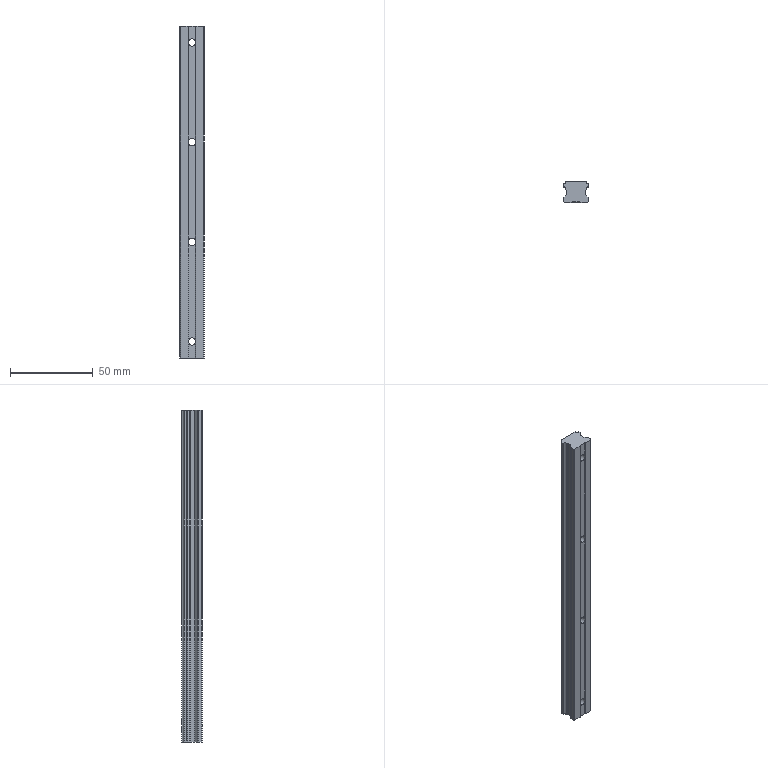Part | STEP file | 11-EG15_RAIL_170CW11 | 1 solid | 70 faces | box 15 x 12.5 x 200 mm | volume 31138 mm3 | cylinder 34 | plane 28 | cone 8 | commonest cylinder face diameters 0.6 x11 4.5 x8 8 x8 3 x5 1 x2